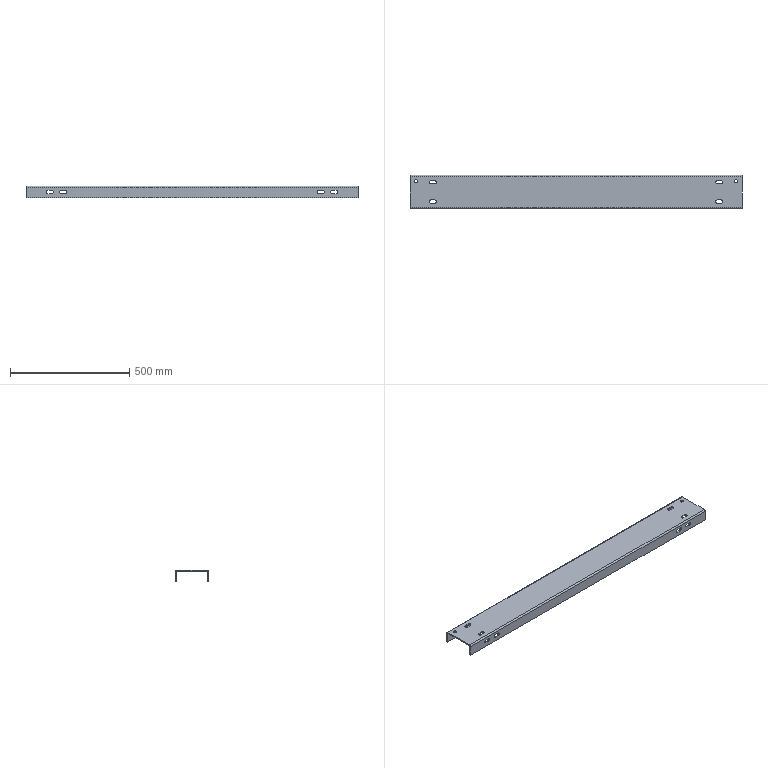Part | 1 solid | 78 faces | box 1390 x 140 x 50 mm | volume 1554100 mm3 | plane 42 | cylinder 36 | commonest cylinder face diameters 13 x16 14 x16 2 x2 12 x2